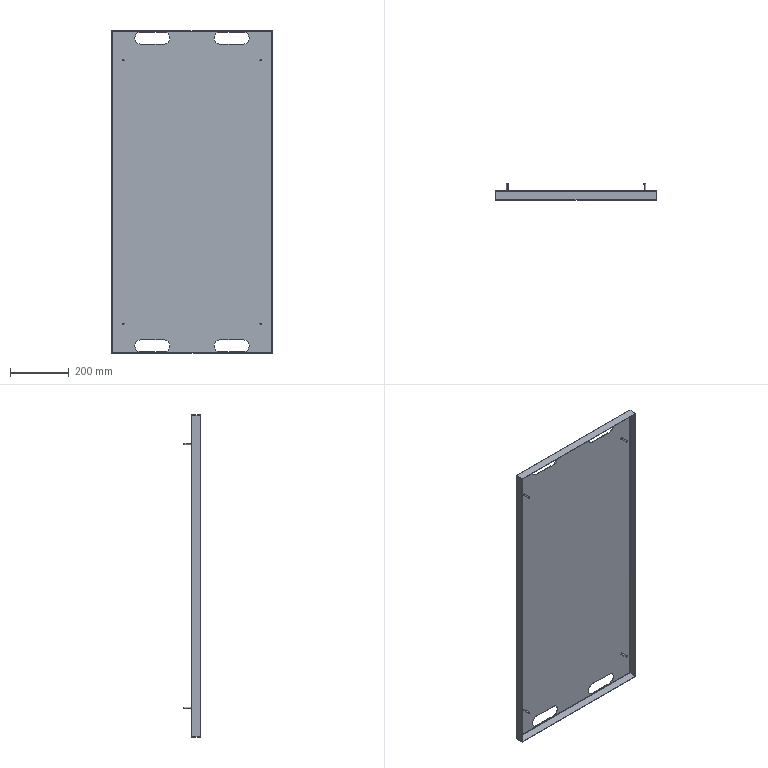Part | SolidWorks | features ICE 2, FlatPattern 1, SMBaseFlange 1, SMMiteredFlange 1, SheetMetal 1 | 1 solid | 78 faces | box 550 x 55 x 1100 mm | volume 1023581 mm3 | plane 38 | cylinder 32 | spline 8 | commonest cylinder face diameters 6 x16 40 x8 1.473 x4 4.473 x4